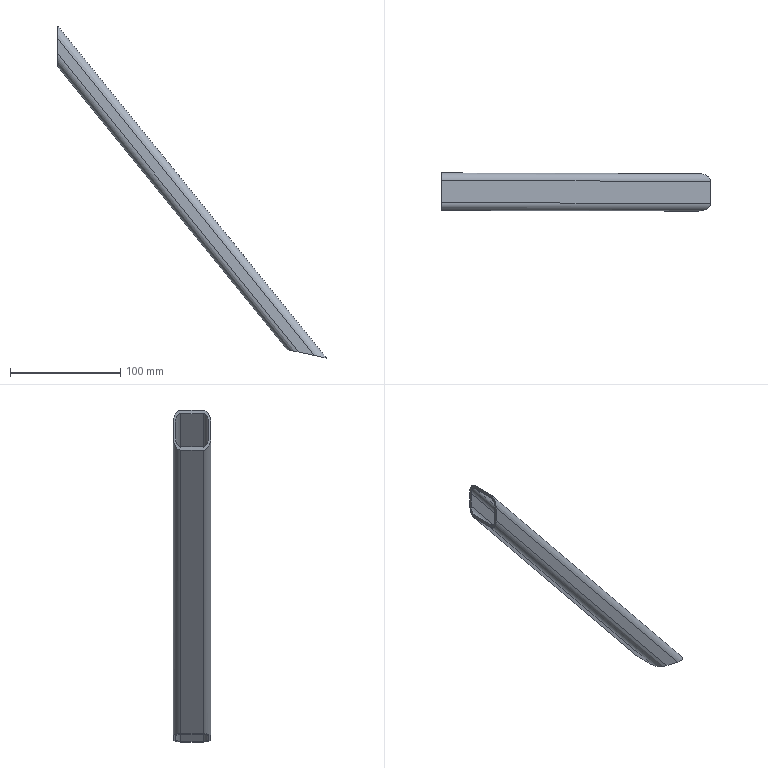Part | STEP file | _model23 | 1 solid | 18 faces | box 243.487 x 34 x 300.682 mm | volume 68472 mm3 | plane 10 | cylinder 8 | commonest cylinder face diameters 10 x4 14 x4